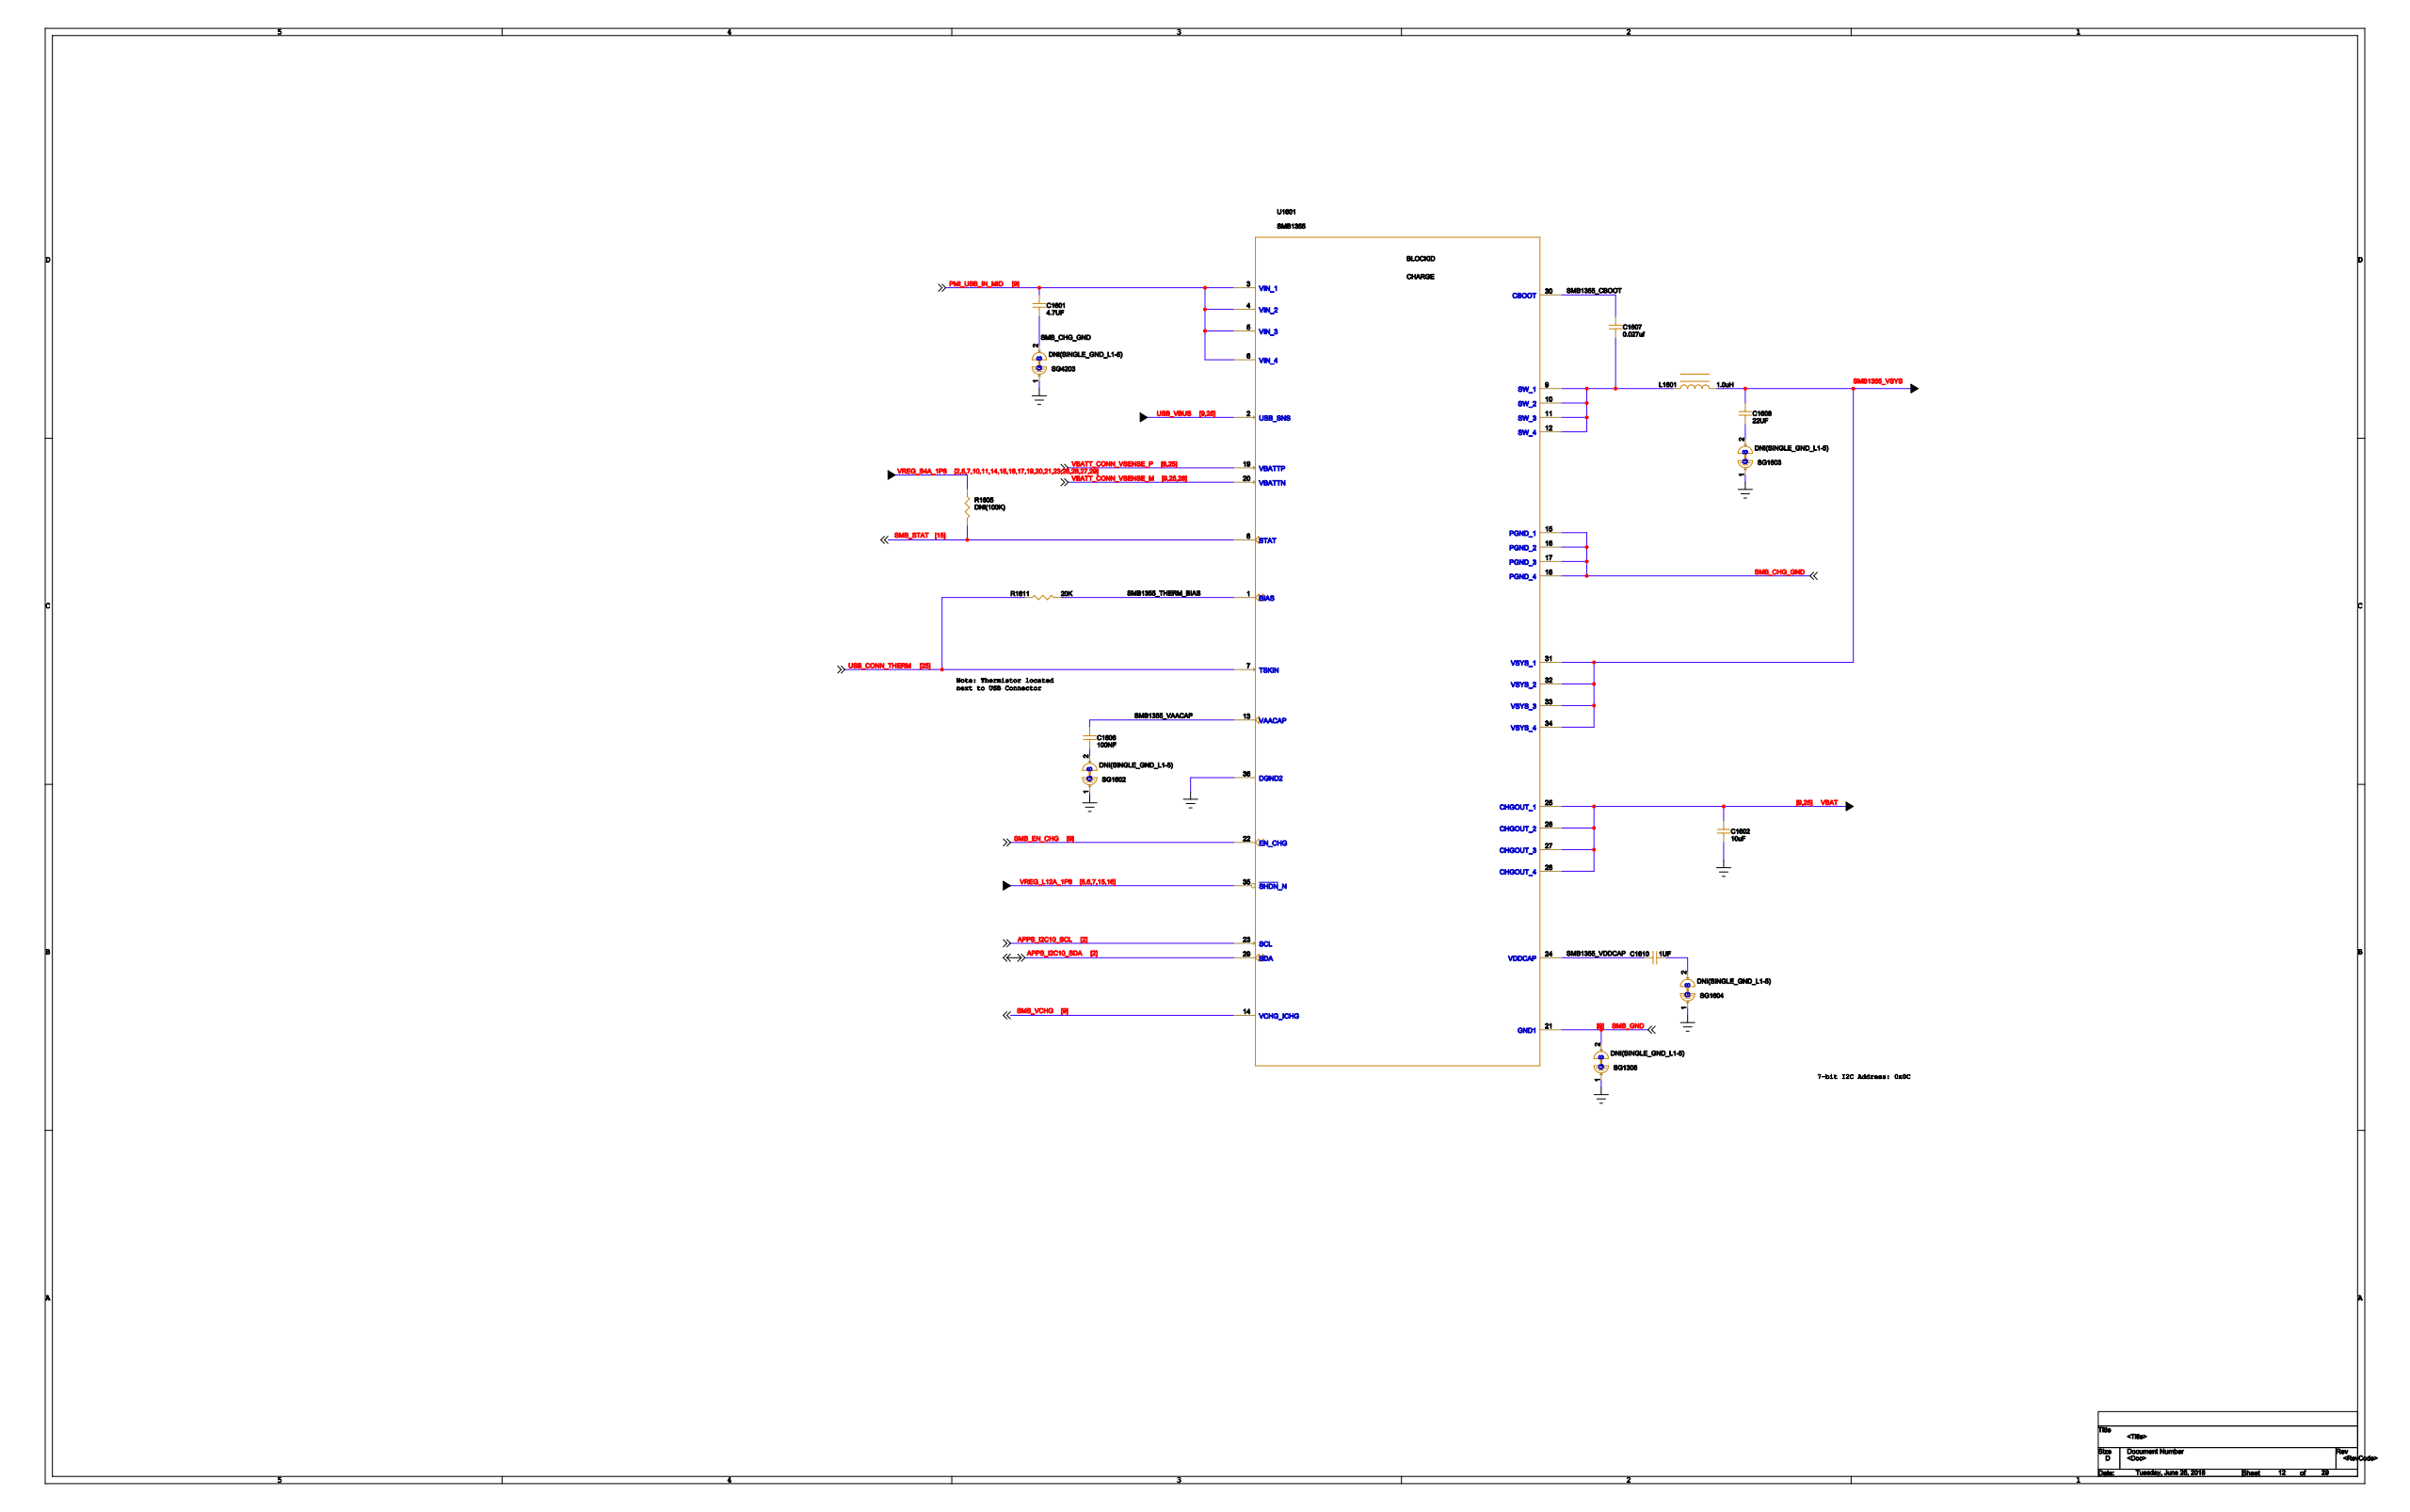Circuit board | Cadence Allegro | 802 parts | 566 nets | one sheet of the schematic
Parts on this sheet (reference | value | footprint):
C1601 | 4.7UF | 0603-BIG
C1602 | 10uF | 0402-BIG
C1606 | 100NF | C0201
C1607 | 0.027uf | 0402-BIG
C1608 | 22UF | 0603-BIG
C1610 | 1uF | C0201
L1601 | 1.0uH | L2520_TFM252008GHM
R1605 | DNI(100K) | R0201
R1611 | 20K | R0201
SG1306 | DNI(SINGLE_GND_L1-5) | GND_L1-5
SG1602 | DNI(SINGLE_GND_L1-5) | GND_L1-5
SG1603 | DNI(SINGLE_GND_L1-5) | GND_L1-5
SG1604 | DNI(SINGLE_GND_L1-5) | GND_L1-5
SG4203 | DNI(SINGLE_GND_L1-5) | GND_L1-5
U1601 | SMB1355 | WLNSP36_2P62X2P62X0P65_0P4
Nets of these parts (net: part-pin ...):
GND: C1602-2 SG1306-1 SG1602-1 SG1603-1 SG1604-1 SG4203-1 U1601-36
VBATT_CONN_VSENSE_P: U1601-19
VBATT_CONN_VSENSE_M: U1601-20
VBAT: C1602-1 U1601-25 U1601-26 U1601-27 U1601-28
USB_VBUS: U1601-2
VREG_S4A_1P8: R1605-1
PMI_USB_IN_MID: C1601-1 U1601-3 U1601-4 U1601-5 U1601-6
SMB1355_VAACAP: C1606-1 U1601-13
N184168: C1606-2 SG1602-2
SMB_STAT: R1605-2 U1601-8
SMB1355_VDDCAP: C1610-1 U1601-24
N183842: C1610-2 SG1604-2
VREG_L12A_1P8: U1601-35
SMB1355_CBOOT: C1607-1 U1601-30
N184094: C1607-2 L1601-1 U1601-9 U1601-10 U1601-11 U1601-12
SMB1355_VSYS: C1608-1 L1601-2 U1601-31 U1601-32 U1601-33 U1601-34
N184452: C1608-2 SG1603-2
SMB_CHG_GND: C1601-2 SG4203-2 U1601-15 U1601-16 U1601-17 U1601-18
APPS_I2C10_SDA: U1601-29
APPS_I2C10_SCL: U1601-23
SMB_EN_CHG: U1601-22
USB_CONN_THERM: R1611-1 U1601-7
SMB1355_THERM_BIAS: R1611-2 U1601-1
SMB_GND: SG1306-2 U1601-21
SMB_VCHG: U1601-14